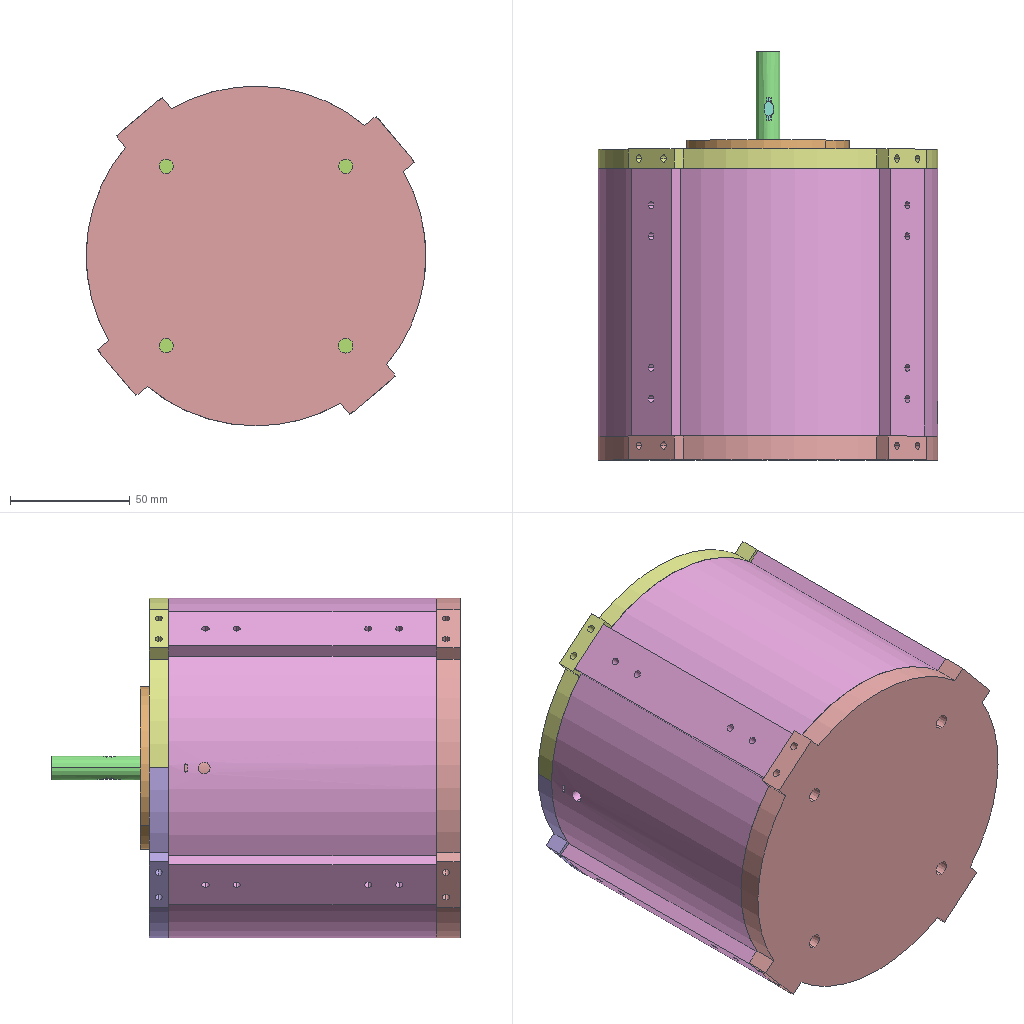Assembly | SolidWorks | 11 different items | 11 placed | box 142 x 171 x 142 mm
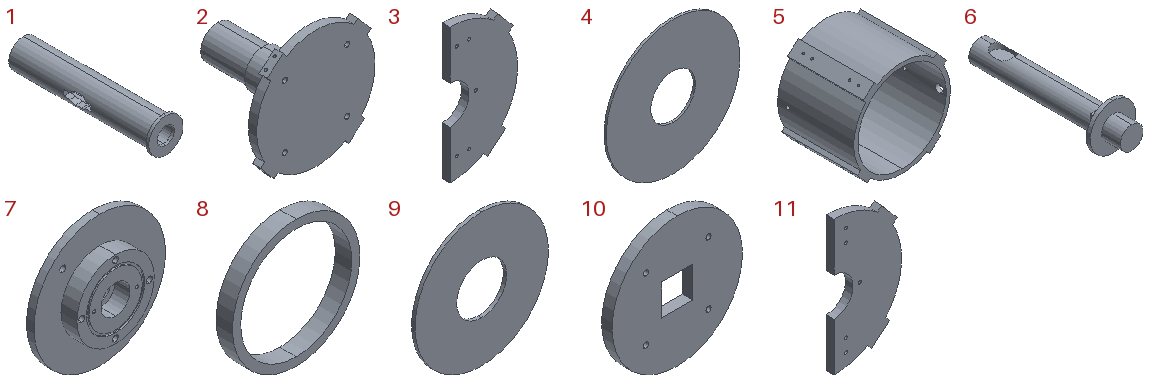Parts list (item | quantity | size | volume | features):
1 | x1 | 12 x 50 x 12 mm | 2925 mm3 | features ICE 3, Revolution 1
2 | x1 | 142 x 118 x 142 mm | 312651 mm3 | features ICE 11, CirPattern 1, RefAxis 1, RevCut 1, Revolution 1
3 | x1 | 71 x 8 x 142 mm | 60040 mm3 | features ICE 4, CirPattern 1, Extrusion 1, RefAxis 1
4 | x1 | 120 x 2 x 120 mm | 20106 mm3 | features Extrusion 1
5 | x1 | 142 x 112 x 142 mm | 337681 mm3 | features ICE 7, CirPattern 1, RefAxis 1, Revolution 1
6 | x1 | 12 x 39.95 x 12 mm | 1172 mm3 | features ICE 4, Revolution 1
7 | x1 | 68 x 12 x 68 mm | 21565 mm3 | features ICE 7, Revolution 2, Extrusion 1, RevCut 1
8 | x1 | 31 x 4 x 31 mm | 728.849 mm3 | features Revolution 1
9 | x1 | 120 x 3 x 120 mm | 29158 mm3 | features Extrusion 1
10 | x1 | 25 x 2 x 25 mm | 903.465 mm3 | features Extrusion 1
11 | x1 | 71 x 8 x 142 mm | 60040 mm3 | features ICE 4, CirPattern 1, Extrusion 1, RefAxis 1
Mates (type | each side: item.copy, entity, surface, feature):
Concentric | 2.1 face cylinder Revolve1 | 4.1 face cylinder Boss-Extrude1
Concentric | 2.1 face cylinder Revolve1 | 9.1 face cylinder Boss-Extrude1
Coincident | 2.1 face plane Revolve1 | 9.1 face plane Boss-Extrude1
Coincident | 2.1 face plane Revolve1 | 4.1 face plane Boss-Extrude1
Concentric | 2.1 face cylinder Revolve1 | 10.1 face cylinder Boss-Extrude1
Concentric | 5.1 face cylinder Revolve1 | 11.1 face cylinder Boss-Extrude1
Concentric | 2.1 face cylinder Revolve1 | 8.1 face cylinder Revolve1
Coincident | 2.1 face plane Cut-Revolve1 | 8.1 face plane Revolve1
DistanceDim | 10.1 face plane Boss-Extrude1 | 2.1 face plane Cut-Revolve1
Coincident | 5.1 face plane Revolve1 | 11.1 face plane Boss-Extrude1
Concentric | 2.1 face cylinder Revolve1 | 5.1 face cylinder Revolve1
Concentric | 6.1 face cylinder Boss-Extrude2 | 1.1 face cylinder Revolve1
Parallel | 6.1 face plane Cut-Extrude2 | 1.1 face plane Cut-Extrude1
Parallel | 6.1 face plane Boss-Extrude1 | 10.1 face plane Boss-Extrude1
Concentric | 6.1 face cylinder Revolve1 | 10.1 face cylinder Boss-Extrude1
Coincident | 6.1 face plane Revolve1 | 10.1 face plane Boss-Extrude1
Coincident | 1.1 face plane Revolve1 | 10.1 face plane Boss-Extrude1
Coincident | 7.1 face plane Boss-Extrude1 | 8.1 face plane Revolve1
Concentric | 5.1 face cylinder Revolve1 | 3.1 face cylinder Boss-Extrude1
Parallel | 11.1 face plane Boss-Extrude1 | 3.1 face plane Boss-Extrude1
Coincident | 5.1 face plane Revolve1 | 3.1 face plane Boss-Extrude1
Coincident | 2.1 face plane Revolve1 | 5.1 face plane Revolve1
Parallel | 5.1 face plane Boss-Extrude3 | 11.1 face plane Boss-Extrude2
Parallel | 2.1 face plane CirPattern2 | 5.1 face plane Boss-Extrude3
Concentric | 7.1 face cylinder Revolve1 | 1.1 face cylinder Revolve1